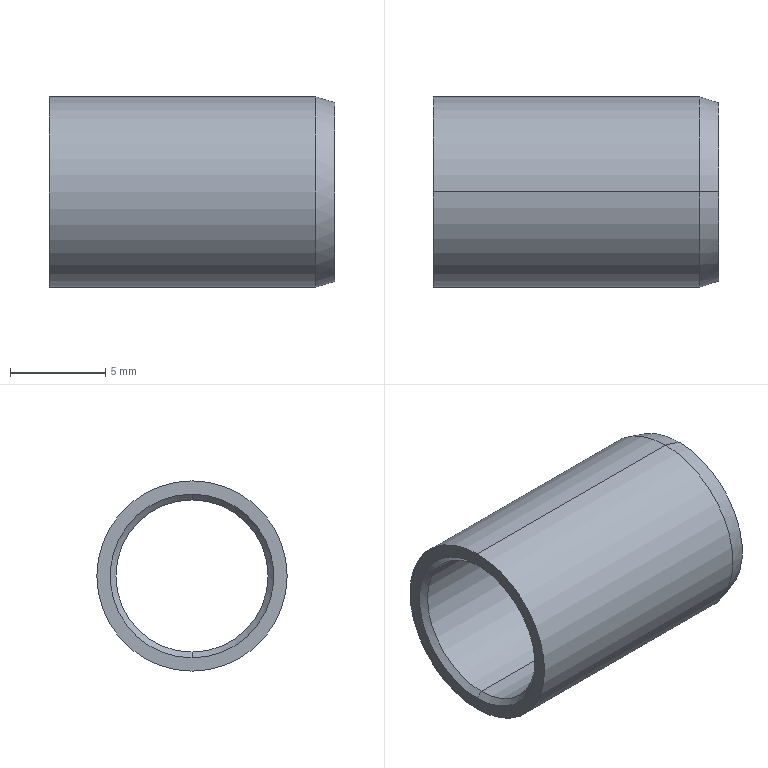Part | STEP file | 0246_001_JZB8-15 | 1 solid | 10 faces | box 15 x 10 x 10 mm | volume 418.338 mm3 | cylinder 4 | cone 4 | plane 2 | commonest cylinder face diameters 8 x2 10 x2
STEP:
#1=CARTESIAN_POINT('',(0.,0.,0.));
#2=DIRECTION('',(0.,0.,1.));
#3=DIRECTION('',(1.,0.,0.));
#4=AXIS2_PLACEMENT_3D('',#1,#2,#3);
#5=CARTESIAN_POINT('',(0.,0.,-5.));
#6=VERTEX_POINT('',#5);
#7=CARTESIAN_POINT('',(0.,0.,5.));
#8=VERTEX_POINT('',#7);
#9=CARTESIAN_POINT('',(0.,0.,0.));
#10=DIRECTION('',(1.,0.,0.));
#11=DIRECTION('',(0.,0.,-1.));
#12=AXIS2_PLACEMENT_3D('',#9,#10,#11);
#13=CIRCLE('',#12,5.);
#14=CARTESIAN_POINT('',(7.,0.,0.));
#15=DIRECTION('',(1.,0.,0.));
#16=DIRECTION('',(0.,0.,-1.));
#17=AXIS2_PLACEMENT_3D('',#14,#15,#16);
#18=CYLINDRICAL_SURFACE('',#17,5.);
#19=CARTESIAN_POINT('',(0.,-7.));
#20=DIRECTION('',(1.,0.));
#21=VECTOR('',#20,1.);
#22=LINE('',#19,#21);
#23=(GEOMETRIC_REPRESENTATION_CONTEXT(2)PARAMETRIC_REPRESENTATION_CONTEXT()REPRESENTATION_CONTEXT('',''));
#24=DEFINITIONAL_REPRESENTATION('',(#22),#23);
#25=PCURVE('',#18,#24);
#26=CARTESIAN_POINT('',(0.,4.65,0.));
#27=DIRECTION('',(-1.,0.,0.));
#28=DIRECTION('',(0.,0.,1.));
#29=AXIS2_PLACEMENT_3D('',#26,#27,#28);
#30=PLANE('',#29);
#31=CARTESIAN_POINT('',(-5.,-4.65));
#32=CARTESIAN_POINT('',(-5.,4.01));
#33=CARTESIAN_POINT('',(2.5,-0.3199));
#34=CARTESIAN_POINT('',(10.,-4.65));
#35=CARTESIAN_POINT('',(2.5,-8.98));
#36=CARTESIAN_POINT('',(-5.,-13.31));
#37=CARTESIAN_POINT('',(-5.,-4.65));
#38=(BOUNDED_CURVE()B_SPLINE_CURVE(2,(#31,#32,#33,#34,#35,#36,#37),.UNSPECIFIED.,.T.,.F.)B_SPLINE_CURVE_WITH_KNOTS((1,2,2,2,2,1),(-2.094,0.,2.094,4.189,6.283,8.378),.UNSPECIFIED.)CURVE()GEOMETRIC_REPRESENTATION_ITEM()RATIONAL_B_SPLINE_CURVE((1.,0.5,1.,0.5,1.,0.5,1.))REPRESENTATION_ITEM(''));
#39=(GEOMETRIC_REPRESENTATION_CONTEXT(2)PARAMETRIC_REPRESENTATION_CONTEXT()REPRESENTATION_CONTEXT('',''));
#40=DEFINITIONAL_REPRESENTATION('',(#38),#39);
#41=PCURVE('',#30,#40);
#42=SURFACE_CURVE('',#13,(#25,#41),.PCURVE_S1.);
#43=EDGE_CURVE('',#6,#8,#42,.T.);
#44=ORIENTED_EDGE('',*,*,#43,.T.);
#45=CARTESIAN_POINT('',(14.,0.,5.));
#46=VERTEX_POINT('',#45);
#47=CARTESIAN_POINT('',(7.,0.,5.));
#48=DIRECTION('',(1.,0.,0.));
#49=VECTOR('',#48,1.);
#50=LINE('',#47,#49);
#51=CARTESIAN_POINT('',(3.142,0.));
#52=DIRECTION('',(0.,1.));
#53=VECTOR('',#52,1.);
#54=LINE('',#51,#53);
#55=(GEOMETRIC_REPRESENTATION_CONTEXT(2)PARAMETRIC_REPRESENTATION_CONTEXT()REPRESENTATION_CONTEXT('',''));
#56=DEFINITIONAL_REPRESENTATION('',(#54),#55);
#57=PCURVE('',#18,#56);
#58=CARTESIAN_POINT('',(7.,0.,0.));
#59=DIRECTION('',(1.,0.,0.));
#60=DIRECTION('',(0.,0.,-1.));
#61=AXIS2_PLACEMENT_3D('',#58,#59,#60);
#62=CYLINDRICAL_SURFACE('',#61,5.);
#63=CARTESIAN_POINT('',(3.142,0.));
#64=DIRECTION('',(0.,1.));
#65=VECTOR('',#64,1.);
#66=LINE('',#63,#65);
#67=(GEOMETRIC_REPRESENTATION_CONTEXT(2)PARAMETRIC_REPRESENTATION_CONTEXT()REPRESENTATION_CONTEXT('',''));
#68=DEFINITIONAL_REPRESENTATION('',(#66),#67);
#69=PCURVE('',#62,#68);
#70=SURFACE_CURVE('',#50,(#57,#69),.PCURVE_S1.);
#71=EDGE_CURVE('',#8,#46,#70,.T.);
#72=ORIENTED_EDGE('',*,*,#71,.T.);
#73=CARTESIAN_POINT('',(14.,0.,-5.));
#74=VERTEX_POINT('',#73);
#75=CARTESIAN_POINT('',(14.,0.,0.));
#76=DIRECTION('',(-1.,0.,0.));
#77=DIRECTION('',(0.,0.,-1.));
#78=AXIS2_PLACEMENT_3D('',#75,#76,#77);
#79=CIRCLE('',#78,5.);
#80=CARTESIAN_POINT('',(6.283,7.));
#81=DIRECTION('',(-1.,0.));
#82=VECTOR('',#81,1.);
#83=LINE('',#80,#82);
#84=(GEOMETRIC_REPRESENTATION_CONTEXT(2)PARAMETRIC_REPRESENTATION_CONTEXT()REPRESENTATION_CONTEXT('',''));
#85=DEFINITIONAL_REPRESENTATION('',(#83),#84);
#86=PCURVE('',#18,#85);
#87=CARTESIAN_POINT('',(14.,0.,0.));
#88=DIRECTION('',(-1.,0.,0.));
#89=DIRECTION('',(0.,0.,1.));
#90=AXIS2_PLACEMENT_3D('',#87,#88,#89);
#91=CONICAL_SURFACE('',#90,5.,0.2915);
#92=CARTESIAN_POINT('',(-3.142,0.));
#93=DIRECTION('',(1.,0.));
#94=VECTOR('',#93,1.);
#95=LINE('',#92,#94);
#96=(GEOMETRIC_REPRESENTATION_CONTEXT(2)PARAMETRIC_REPRESENTATION_CONTEXT()REPRESENTATION_CONTEXT('',''));
#97=DEFINITIONAL_REPRESENTATION('',(#95),#96);
#98=PCURVE('',#91,#97);
#99=SURFACE_CURVE('',#79,(#86,#98),.PCURVE_S1.);
#100=EDGE_CURVE('',#46,#74,#99,.T.);
#101=ORIENTED_EDGE('',*,*,#100,.T.);
#102=CARTESIAN_POINT('',(7.,0.,-5.));
#103=DIRECTION('',(1.,0.,0.));
#104=VECTOR('',#103,1.);
#105=LINE('',#102,#104);
#106=CARTESIAN_POINT('',(0.,0.));
#107=DIRECTION('',(0.,1.));
#108=VECTOR('',#107,1.);
#109=LINE('',#106,#108);
#110=(GEOMETRIC_REPRESENTATION_CONTEXT(2)PARAMETRIC_REPRESENTATION_CONTEXT()REPRESENTATION_CONTEXT('',''));
#111=DEFINITIONAL_REPRESENTATION('',(#109),#110);
#112=PCURVE('',#18,#111);
#113=CARTESIAN_POINT('',(6.283,0.));
#114=DIRECTION('',(0.,1.));
#115=VECTOR('',#114,1.);
#116=LINE('',#113,#115);
#117=(GEOMETRIC_REPRESENTATION_CONTEXT(2)PARAMETRIC_REPRESENTATION_CONTEXT()REPRESENTATION_CONTEXT('',''));
#118=DEFINITIONAL_REPRESENTATION('',(#116),#117);
#119=PCURVE('',#62,#118);
#120=SURFACE_CURVE('',#105,(#112,#119),.PCURVE_S1.);
#121=EDGE_CURVE('',#6,#74,#120,.T.);
#122=ORIENTED_EDGE('',*,*,#121,.F.);
#123=EDGE_LOOP('',(#44,#72,#101,#122));
#124=FACE_BOUND('',#123,.T.);
#125=ADVANCED_FACE('',(#124),#18,.T.);
#126=CARTESIAN_POINT('',(15.,0.,4.7));
#127=VERTEX_POINT('',#126);
#128=CARTESIAN_POINT('',(15.,0.,-4.7));
#129=VERTEX_POINT('',#128);
#130=CARTESIAN_POINT('',(15.,0.,0.));
#131=DIRECTION('',(-1.,0.,0.));
#132=DIRECTION('',(0.,0.,1.));
#133=AXIS2_PLACEMENT_3D('',#130,#131,#132);
#134=CIRCLE('',#133,4.7);
#135=CARTESIAN_POINT('',(0.,-1.));
#136=DIRECTION('',(1.,0.));
#137=VECTOR('',#136,1.);
#138=LINE('',#135,#137);
#139=(GEOMETRIC_REPRESENTATION_CONTEXT(2)PARAMETRIC_REPRESENTATION_CONTEXT()REPRESENTATION_CONTEXT('',''));
#140=DEFINITIONAL_REPRESENTATION('',(#138),#139);
#141=PCURVE('',#91,#140);
#142=CARTESIAN_POINT('',(15.,4.35,0.));
#143=DIRECTION('',(1.,0.,0.));
#144=DIRECTION('',(0.,0.,-1.));
#145=AXIS2_PLACEMENT_3D('',#142,#143,#144);
#146=PLANE('',#145);
#147=CARTESIAN_POINT('',(-4.7,-4.35));
#148=CARTESIAN_POINT('',(-4.7,3.791));
#149=CARTESIAN_POINT('',(2.35,-0.2797));
#150=CARTESIAN_POINT('',(9.4,-4.35));
#151=CARTESIAN_POINT('',(2.35,-8.42));
#152=CARTESIAN_POINT('',(-4.7,-12.491));
#153=CARTESIAN_POINT('',(-4.7,-4.35));
#154=(BOUNDED_CURVE()B_SPLINE_CURVE(2,(#147,#148,#149,#150,#151,#152,#153),.UNSPECIFIED.,.T.,.F.)B_SPLINE_CURVE_WITH_KNOTS((1,2,2,2,2,1),(-2.094,0.,2.094,4.189,6.283,8.378),.UNSPECIFIED.)CURVE()GEOMETRIC_REPRESENTATION_ITEM()RATIONAL_B_SPLINE_CURVE((1.,0.5,1.,0.5,1.,0.5,1.))REPRESENTATION_ITEM(''));
#155=(GEOMETRIC_REPRESENTATION_CONTEXT(2)PARAMETRIC_REPRESENTATION_CONTEXT()REPRESENTATION_CONTEXT('',''));
#156=DEFINITIONAL_REPRESENTATION('',(#154),#155);
#157=PCURVE('',#146,#156);
#158=SURFACE_CURVE('',#134,(#141,#157),.PCURVE_S1.);
#159=EDGE_CURVE('',#127,#129,#158,.T.);
#160=ORIENTED_EDGE('',*,*,#159,.T.);
#161=CARTESIAN_POINT('',(14.,0.,-5.));
#162=DIRECTION('',(-0.9578,0.,-0.2873));
#163=VECTOR('',#162,1.);
#164=LINE('',#161,#163);
#165=CARTESIAN_POINT('',(3.142,0.));
#166=DIRECTION('',(0.,1.));
#167=VECTOR('',#166,1.);
#168=LINE('',#165,#167);
#169=(GEOMETRIC_REPRESENTATION_CONTEXT(2)PARAMETRIC_REPRESENTATION_CONTEXT()REPRESENTATION_CONTEXT('',''));
#170=DEFINITIONAL_REPRESENTATION('',(#168),#169);
#171=PCURVE('',#91,#170);
#172=CARTESIAN_POINT('',(14.,0.,0.));
#173=DIRECTION('',(-1.,0.,0.));
#174=DIRECTION('',(0.,0.,1.));
#175=AXIS2_PLACEMENT_3D('',#172,#173,#174);
#176=CONICAL_SURFACE('',#175,5.,0.2915);
#177=CARTESIAN_POINT('',(3.142,0.));
#178=DIRECTION('',(0.,1.));
#179=VECTOR('',#178,1.);
#180=LINE('',#177,#179);
#181=(GEOMETRIC_REPRESENTATION_CONTEXT(2)PARAMETRIC_REPRESENTATION_CONTEXT()REPRESENTATION_CONTEXT('',''));
#182=DEFINITIONAL_REPRESENTATION('',(#180),#181);
#183=PCURVE('',#176,#182);
#184=SURFACE_CURVE('',#164,(#171,#183),.PCURVE_S1.);
#185=EDGE_CURVE('',#129,#74,#184,.T.);
#186=ORIENTED_EDGE('',*,*,#185,.T.);
#187=ORIENTED_EDGE('',*,*,#100,.F.);
#188=CARTESIAN_POINT('',(14.,0.,5.));
#189=DIRECTION('',(-0.9578,0.,0.2873));
#190=VECTOR('',#189,1.);
#191=LINE('',#188,#190);
#192=CARTESIAN_POINT('',(0.,0.));
#193=DIRECTION('',(0.,1.));
#194=VECTOR('',#193,1.);
#195=LINE('',#192,#194);
#196=(GEOMETRIC_REPRESENTATION_CONTEXT(2)PARAMETRIC_REPRESENTATION_CONTEXT()REPRESENTATION_CONTEXT('',''));
#197=DEFINITIONAL_REPRESENTATION('',(#195),#196);
#198=PCURVE('',#91,#197);
#199=CARTESIAN_POINT('',(6.283,0.));
#200=DIRECTION('',(0.,1.));
#201=VECTOR('',#200,1.);
#202=LINE('',#199,#201);
#203=(GEOMETRIC_REPRESENTATION_CONTEXT(2)PARAMETRIC_REPRESENTATION_CONTEXT()REPRESENTATION_CONTEXT('',''));
#204=DEFINITIONAL_REPRESENTATION('',(#202),#203);
#205=PCURVE('',#176,#204);
#206=SURFACE_CURVE('',#191,(#198,#205),.PCURVE_S1.);
#207=EDGE_CURVE('',#127,#46,#206,.T.);
#208=ORIENTED_EDGE('',*,*,#207,.F.);
#209=EDGE_LOOP('',(#160,#186,#187,#208));
#210=FACE_BOUND('',#209,.T.);
#211=ADVANCED_FACE('',(#210),#91,.T.);
#212=CARTESIAN_POINT('',(0.3,0.,4.));
#213=VERTEX_POINT('',#212);
#214=CARTESIAN_POINT('',(0.,0.,4.3));
#215=VERTEX_POINT('',#214);
#216=CARTESIAN_POINT('',(0.,0.,4.3));
#217=DIRECTION('',(-0.7071,0.,0.7071));
#218=VECTOR('',#217,1.);
#219=LINE('',#216,#218);
#220=CARTESIAN_POINT('',(0.,0.,0.));
#221=DIRECTION('',(-1.,0.,0.));
#222=DIRECTION('',(0.,0.,1.));
#223=AXIS2_PLACEMENT_3D('',#220,#221,#222);
#224=CONICAL_SURFACE('',#223,4.3,0.7854);
#225=CARTESIAN_POINT('',(6.283,0.));
#226=DIRECTION('',(0.,1.));
#227=VECTOR('',#226,1.);
#228=LINE('',#225,#227);
#229=(GEOMETRIC_REPRESENTATION_CONTEXT(2)PARAMETRIC_REPRESENTATION_CONTEXT()REPRESENTATION_CONTEXT('',''));
#230=DEFINITIONAL_REPRESENTATION('',(#228),#229);
#231=PCURVE('',#224,#230);
#232=CARTESIAN_POINT('',(0.,0.,0.));
#233=DIRECTION('',(-1.,0.,0.));
#234=DIRECTION('',(0.,0.,1.));
#235=AXIS2_PLACEMENT_3D('',#232,#233,#234);
#236=CONICAL_SURFACE('',#235,4.3,0.7854);
#237=CARTESIAN_POINT('',(0.,0.));
#238=DIRECTION('',(0.,1.));
#239=VECTOR('',#238,1.);
#240=LINE('',#237,#239);
#241=(GEOMETRIC_REPRESENTATION_CONTEXT(2)PARAMETRIC_REPRESENTATION_CONTEXT()REPRESENTATION_CONTEXT('',''));
#242=DEFINITIONAL_REPRESENTATION('',(#240),#241);
#243=PCURVE('',#236,#242);
#244=SURFACE_CURVE('',#219,(#231,#243),.PCURVE_S1.);
#245=EDGE_CURVE('',#213,#215,#244,.T.);
#246=ORIENTED_EDGE('',*,*,#245,.T.);
#247=CARTESIAN_POINT('',(0.,0.,-4.3));
#248=VERTEX_POINT('',#247);
#249=CARTESIAN_POINT('',(0.,0.,0.));
#250=DIRECTION('',(1.,0.,0.));
#251=DIRECTION('',(0.,0.,1.));
#252=AXIS2_PLACEMENT_3D('',#249,#250,#251);
#253=CIRCLE('',#252,4.3);
#254=CARTESIAN_POINT('',(6.283,0.));
#255=DIRECTION('',(-1.,0.));
#256=VECTOR('',#255,1.);
#257=LINE('',#254,#256);
#258=(GEOMETRIC_REPRESENTATION_CONTEXT(2)PARAMETRIC_REPRESENTATION_CONTEXT()REPRESENTATION_CONTEXT('',''));
#259=DEFINITIONAL_REPRESENTATION('',(#257),#258);
#260=PCURVE('',#224,#259);
#261=CARTESIAN_POINT('',(4.3,-4.65));
#262=CARTESIAN_POINT('',(4.3,-12.098));
#263=CARTESIAN_POINT('',(-2.15,-8.374));
#264=CARTESIAN_POINT('',(-8.6,-4.65));
#265=CARTESIAN_POINT('',(-2.15,-0.9261));
#266=CARTESIAN_POINT('',(4.3,2.798));
#267=CARTESIAN_POINT('',(4.3,-4.65));
#268=(BOUNDED_CURVE()B_SPLINE_CURVE(2,(#261,#262,#263,#264,#265,#266,#267),.UNSPECIFIED.,.T.,.F.)B_SPLINE_CURVE_WITH_KNOTS((1,2,2,2,2,1),(-2.094,0.,2.094,4.189,6.283,8.378),.UNSPECIFIED.)CURVE()GEOMETRIC_REPRESENTATION_ITEM()RATIONAL_B_SPLINE_CURVE((1.,0.5,1.,0.5,1.,0.5,1.))REPRESENTATION_ITEM(''));
#269=(GEOMETRIC_REPRESENTATION_CONTEXT(2)PARAMETRIC_REPRESENTATION_CONTEXT()REPRESENTATION_CONTEXT('',''));
#270=DEFINITIONAL_REPRESENTATION('',(#268),#269);
#271=PCURVE('',#30,#270);
#272=SURFACE_CURVE('',#253,(#260,#271),.PCURVE_S1.);
#273=EDGE_CURVE('',#215,#248,#272,.T.);
#274=ORIENTED_EDGE('',*,*,#273,.T.);
#275=CARTESIAN_POINT('',(0.3,0.,-4.));
#276=VERTEX_POINT('',#275);
#277=CARTESIAN_POINT('',(0.,0.,-4.3));
#278=DIRECTION('',(-0.7071,0.,-0.7071));
#279=VECTOR('',#278,1.);
#280=LINE('',#277,#279);
#281=CARTESIAN_POINT('',(3.142,0.));
#282=DIRECTION('',(0.,1.));
#283=VECTOR('',#282,1.);
#284=LINE('',#281,#283);
#285=(GEOMETRIC_REPRESENTATION_CONTEXT(2)PARAMETRIC_REPRESENTATION_CONTEXT()REPRESENTATION_CONTEXT('',''));
#286=DEFINITIONAL_REPRESENTATION('',(#284),#285);
#287=PCURVE('',#224,#286);
#288=CARTESIAN_POINT('',(3.142,0.));
#289=DIRECTION('',(0.,1.));
#290=VECTOR('',#289,1.);
#291=LINE('',#288,#290);
#292=(GEOMETRIC_REPRESENTATION_CONTEXT(2)PARAMETRIC_REPRESENTATION_CONTEXT()REPRESENTATION_CONTEXT('',''));
#293=DEFINITIONAL_REPRESENTATION('',(#291),#292);
#294=PCURVE('',#236,#293);
#295=SURFACE_CURVE('',#280,(#287,#294),.PCURVE_S1.);
#296=EDGE_CURVE('',#276,#248,#295,.T.);
#297=ORIENTED_EDGE('',*,*,#296,.F.);
#298=CARTESIAN_POINT('',(0.3,0.,0.));
#299=DIRECTION('',(-1.,0.,0.));
#300=DIRECTION('',(0.,1.,0.));
#301=AXIS2_PLACEMENT_3D('',#298,#299,#300);
#302=CIRCLE('',#301,4.);
#303=CARTESIAN_POINT('',(1.571,-0.3));
#304=DIRECTION('',(1.,0.));
#305=VECTOR('',#304,1.);
#306=LINE('',#303,#305);
#307=(GEOMETRIC_REPRESENTATION_CONTEXT(2)PARAMETRIC_REPRESENTATION_CONTEXT()REPRESENTATION_CONTEXT('',''));
#308=DEFINITIONAL_REPRESENTATION('',(#306),#307);
#309=PCURVE('',#224,#308);
#310=CARTESIAN_POINT('',(7.65,0.,0.));
#311=DIRECTION('',(1.,0.,0.));
#312=DIRECTION('',(0.,0.,-1.));
#313=AXIS2_PLACEMENT_3D('',#310,#311,#312);
#314=CYLINDRICAL_SURFACE('',#313,4.);
#315=CARTESIAN_POINT('',(7.854,-7.35));
#316=DIRECTION('',(-1.,0.));
#317=VECTOR('',#316,1.);
#318=LINE('',#315,#317);
#319=(GEOMETRIC_REPRESENTATION_CONTEXT(2)PARAMETRIC_REPRESENTATION_CONTEXT()REPRESENTATION_CONTEXT('',''));
#320=DEFINITIONAL_REPRESENTATION('',(#318),#319);
#321=PCURVE('',#314,#320);
#322=SURFACE_CURVE('',#302,(#309,#321),.PCURVE_S1.);
#323=EDGE_CURVE('',#276,#213,#322,.T.);
#324=ORIENTED_EDGE('',*,*,#323,.T.);
#325=EDGE_LOOP('',(#246,#274,#297,#324));
#326=FACE_BOUND('',#325,.F.);
#327=ADVANCED_FACE('',(#326),#224,.F.);
#328=CARTESIAN_POINT('',(15.,0.,-4.));
#329=VERTEX_POINT('',#328);
#330=CARTESIAN_POINT('',(7.65,0.,-4.));
#331=DIRECTION('',(1.,0.,0.));
#332=VECTOR('',#331,1.);
#333=LINE('',#330,#332);
#334=CARTESIAN_POINT('',(6.283,0.));
#335=DIRECTION('',(0.,1.));
#336=VECTOR('',#335,1.);
#337=LINE('',#334,#336);
#338=(GEOMETRIC_REPRESENTATION_CONTEXT(2)PARAMETRIC_REPRESENTATION_CONTEXT()REPRESENTATION_CONTEXT('',''));
#339=DEFINITIONAL_REPRESENTATION('',(#337),#338);
#340=PCURVE('',#314,#339);
#341=CARTESIAN_POINT('',(7.65,0.,0.));
#342=DIRECTION('',(1.,0.,0.));
#343=DIRECTION('',(0.,0.,-1.));
#344=AXIS2_PLACEMENT_3D('',#341,#342,#343);
#345=CYLINDRICAL_SURFACE('',#344,4.);
#346=CARTESIAN_POINT('',(0.,0.));
#347=DIRECTION('',(0.,1.));
#348=VECTOR('',#347,1.);
#349=LINE('',#346,#348);
#350=(GEOMETRIC_REPRESENTATION_CONTEXT(2)PARAMETRIC_REPRESENTATION_CONTEXT()REPRESENTATION_CONTEXT('',''));
#351=DEFINITIONAL_REPRESENTATION('',(#349),#350);
#352=PCURVE('',#345,#351);
#353=SURFACE_CURVE('',#333,(#340,#352),.PCURVE_S1.);
#354=EDGE_CURVE('',#276,#329,#353,.T.);
#355=ORIENTED_EDGE('',*,*,#354,.T.);
#356=CARTESIAN_POINT('',(15.,0.,4.));
#357=VERTEX_POINT('',#356);
#358=CARTESIAN_POINT('',(15.,0.,0.));
#359=DIRECTION('',(-1.,0.,0.));
#360=DIRECTION('',(0.,0.,-1.));
#361=AXIS2_PLACEMENT_3D('',#358,#359,#360);
#362=CIRCLE('',#361,4.);
#363=CARTESIAN_POINT('',(6.283,7.35));
#364=DIRECTION('',(-1.,0.));
#365=VECTOR('',#364,1.);
#366=LINE('',#363,#365);
#367=(GEOMETRIC_REPRESENTATION_CONTEXT(2)PARAMETRIC_REPRESENTATION_CONTEXT()REPRESENTATION_CONTEXT('',''));
#368=DEFINITIONAL_REPRESENTATION('',(#366),#367);
#369=PCURVE('',#314,#368);
#370=CARTESIAN_POINT('',(4.,-4.35));
#371=CARTESIAN_POINT('',(4.,-11.278));
#372=CARTESIAN_POINT('',(-2.,-7.814));
#373=CARTESIAN_POINT('',(-8.,-4.35));
#374=CARTESIAN_POINT('',(-2.,-0.8859));
#375=CARTESIAN_POINT('',(4.,2.578));
#376=CARTESIAN_POINT('',(4.,-4.35));
#377=(BOUNDED_CURVE()B_SPLINE_CURVE(2,(#370,#371,#372,#373,#374,#375,#376),.UNSPECIFIED.,.T.,.F.)B_SPLINE_CURVE_WITH_KNOTS((1,2,2,2,2,1),(-2.094,0.,2.094,4.189,6.283,8.378),.UNSPECIFIED.)CURVE()GEOMETRIC_REPRESENTATION_ITEM()RATIONAL_B_SPLINE_CURVE((1.,0.5,1.,0.5,1.,0.5,1.))REPRESENTATION_ITEM(''));
#378=(GEOMETRIC_REPRESENTATION_CONTEXT(2)PARAMETRIC_REPRESENTATION_CONTEXT()REPRESENTATION_CONTEXT('',''));
#379=DEFINITIONAL_REPRESENTATION('',(#377),#378);
#380=PCURVE('',#146,#379);
#381=SURFACE_CURVE('',#362,(#369,#380),.PCURVE_S1.);
#382=EDGE_CURVE('',#329,#357,#381,.T.);
#383=ORIENTED_EDGE('',*,*,#382,.T.);
#384=CARTESIAN_POINT('',(7.65,0.,4.));
#385=DIRECTION('',(1.,0.,0.));
#386=VECTOR('',#385,1.);
#387=LINE('',#384,#386);
#388=CARTESIAN_POINT('',(3.142,0.));
#389=DIRECTION('',(0.,1.));
#390=VECTOR('',#389,1.);
#391=LINE('',#388,#390);
#392=(GEOMETRIC_REPRESENTATION_CONTEXT(2)PARAMETRIC_REPRESENTATION_CONTEXT()REPRESENTATION_CONTEXT('',''));
#393=DEFINITIONAL_REPRESENTATION('',(#391),#392);
#394=PCURVE('',#314,#393);
#395=CARTESIAN_POINT('',(3.142,0.));
#396=DIRECTION('',(0.,1.));
#397=VECTOR('',#396,1.);
#398=LINE('',#395,#397);
#399=(GEOMETRIC_REPRESENTATION_CONTEXT(2)PARAMETRIC_REPRESENTATION_CONTEXT()REPRESENTATION_CONTEXT('',''));
#400=DEFINITIONAL_REPRESENTATION('',(#398),#399);
#401=PCURVE('',#345,#400);
#402=SURFACE_CURVE('',#387,(#394,#401),.PCURVE_S1.);
#403=EDGE_CURVE('',#213,#357,#402,.T.);
#404=ORIENTED_EDGE('',*,*,#403,.F.);
#405=ORIENTED_EDGE('',*,*,#323,.F.);
#406=EDGE_LOOP('',(#355,#383,#404,#405));
#407=FACE_BOUND('',#406,.F.);
#408=ADVANCED_FACE('',(#407),#314,.F.);
#409=ORIENTED_EDGE('',*,*,#71,.F.);
#410=CARTESIAN_POINT('',(0.,0.,0.));
#411=DIRECTION('',(1.,0.,0.));
#412=DIRECTION('',(0.,0.,-1.));
#413=AXIS2_PLACEMENT_3D('',#410,#411,#412);
#414=CIRCLE('',#413,5.);
#415=CARTESIAN_POINT('',(0.,-7.));
#416=DIRECTION('',(1.,0.));
#417=VECTOR('',#416,1.);
#418=LINE('',#415,#417);
#419=(GEOMETRIC_REPRESENTATION_CONTEXT(2)PARAMETRIC_REPRESENTATION_CONTEXT()REPRESENTATION_CONTEXT('',''));
#420=DEFINITIONAL_REPRESENTATION('',(#418),#419);
#421=PCURVE('',#62,#420);
#422=CARTESIAN_POINT('',(-5.,-4.65));
#423=CARTESIAN_POINT('',(-5.,4.01));
#424=CARTESIAN_POINT('',(2.5,-0.3199));
#425=CARTESIAN_POINT('',(10.,-4.65));
#426=CARTESIAN_POINT('',(2.5,-8.98));
#427=CARTESIAN_POINT('',(-5.,-13.31));
#428=CARTESIAN_POINT('',(-5.,-4.65));
#429=(BOUNDED_CURVE()B_SPLINE_CURVE(2,(#422,#423,#424,#425,#426,#427,#428),.UNSPECIFIED.,.T.,.F.)B_SPLINE_CURVE_WITH_KNOTS((1,2,2,2,2,1),(-2.094,0.,2.094,4.189,6.283,8.378),.UNSPECIFIED.)CURVE()GEOMETRIC_REPRESENTATION_ITEM()RATIONAL_B_SPLINE_CURVE((1.,0.5,1.,0.5,1.,0.5,1.))REPRESENTATION_ITEM(''));
#430=(GEOMETRIC_REPRESENTATION_CONTEXT(2)PARAMETRIC_REPRESENTATION_CONTEXT()REPRESENTATION_CONTEXT('',''));
#431=DEFINITIONAL_REPRESENTATION('',(#429),#430);
#432=PCURVE('',#30,#431);
#433=SURFACE_CURVE('',#414,(#421,#432),.PCURVE_S1.);
#434=EDGE_CURVE('',#8,#6,#433,.T.);
#435=ORIENTED_EDGE('',*,*,#434,.T.);
#436=ORIENTED_EDGE('',*,*,#121,.T.);
#437=CARTESIAN_POINT('',(14.,0.,0.));
#438=DIRECTION('',(-1.,0.,0.));
#439=DIRECTION('',(0.,0.,-1.));
#440=AXIS2_PLACEMENT_3D('',#437,#438,#439);
#441=CIRCLE('',#440,5.);
#442=CARTESIAN_POINT('',(6.283,7.));
#443=DIRECTION('',(-1.,0.));
#444=VECTOR('',#443,1.);
#445=LINE('',#442,#444);
#446=(GEOMETRIC_REPRESENTATION_CONTEXT(2)PARAMETRIC_REPRESENTATION_CONTEXT()REPRESENTATION_CONTEXT('',''));
#447=DEFINITIONAL_REPRESENTATION('',(#445),#446);
#448=PCURVE('',#62,#447);
#449=CARTESIAN_POINT('',(3.142,0.));
#450=DIRECTION('',(1.,0.));
#451=VECTOR('',#450,1.);
#452=LINE('',#449,#451);
#453=(GEOMETRIC_REPRESENTATION_CONTEXT(2)PARAMETRIC_REPRESENTATION_CONTEXT()REPRESENTATION_CONTEXT('',''));
#454=DEFINITIONAL_REPRESENTATION('',(#452),#453);
#455=PCURVE('',#176,#454);
#456=SURFACE_CURVE('',#441,(#448,#455),.PCURVE_S1.);
#457=EDGE_CURVE('',#74,#46,#456,.T.);
#458=ORIENTED_EDGE('',*,*,#457,.T.);
#459=EDGE_LOOP('',(#409,#435,#436,#458));
#460=FACE_BOUND('',#459,.T.);
#461=ADVANCED_FACE('',(#460),#62,.T.);
#462=ORIENTED_EDGE('',*,*,#43,.F.);
#463=ORIENTED_EDGE('',*,*,#434,.F.);
#464=EDGE_LOOP('',(#462,#463));
#465=FACE_BOUND('',#464,.T.);
#466=ORIENTED_EDGE('',*,*,#273,.T.);
#467=CARTESIAN_POINT('',(0.,0.,0.));
#468=DIRECTION('',(1.,0.,0.));
#469=DIRECTION('',(0.,0.,1.));
#470=AXIS2_PLACEMENT_3D('',#467,#468,#469);
#471=CIRCLE('',#470,4.3);
#472=CARTESIAN_POINT('',(4.3,-4.65));
#473=CARTESIAN_POINT('',(4.3,-12.098));
#474=CARTESIAN_POINT('',(-2.15,-8.374));
#475=CARTESIAN_POINT('',(-8.6,-4.65));
#476=CARTESIAN_POINT('',(-2.15,-0.9261));
#477=CARTESIAN_POINT('',(4.3,2.798));
#478=CARTESIAN_POINT('',(4.3,-4.65));
#479=(BOUNDED_CURVE()B_SPLINE_CURVE(2,(#472,#473,#474,#475,#476,#477,#478),.UNSPECIFIED.,.T.,.F.)B_SPLINE_CURVE_WITH_KNOTS((1,2,2,2,2,1),(-2.094,0.,2.094,4.189,6.283,8.378),.UNSPECIFIED.)CURVE()GEOMETRIC_REPRESENTATION_ITEM()RATIONAL_B_SPLINE_CURVE((1.,0.5,1.,0.5,1.,0.5,1.))REPRESENTATION_ITEM(''));
#480=(GEOMETRIC_REPRESENTATION_CONTEXT(2)PARAMETRIC_REPRESENTATION_CONTEXT()REPRESENTATION_CONTEXT('',''));
#481=DEFINITIONAL_REPRESENTATION('',(#479),#480);
#482=PCURVE('',#30,#481);
#483=CARTESIAN_POINT('',(6.283,0.));
#484=DIRECTION('',(-1.,0.));
#485=VECTOR('',#484,1.);
#486=LINE('',#483,#485);
#487=(GEOMETRIC_REPRESENTATION_CONTEXT(2)PARAMETRIC_REPRESENTATION_CONTEXT()REPRESENTATION_CONTEXT('',''));
#488=DEFINITIONAL_REPRESENTATION('',(#486),#487);
#489=PCURVE('',#236,#488);
#490=SURFACE_CURVE('',#471,(#482,#489),.PCURVE_S1.);
#491=EDGE_CURVE('',#248,#215,#490,.T.);
#492=ORIENTED_EDGE('',*,*,#491,.T.);
#493=EDGE_LOOP('',(#466,#492));
#494=FACE_BOUND('',#493,.T.);
#495=ADVANCED_FACE('',(#465,#494),#30,.T.);
#496=ORIENTED_EDGE('',*,*,#185,.F.);
#497=CARTESIAN_POINT('',(15.,0.,0.));
#498=DIRECTION('',(-1.,0.,0.));
#499=DIRECTION('',(0.,0.,1.));
#500=AXIS2_PLACEMENT_3D('',#497,#498,#499);
#501=CIRCLE('',#500,4.7);
#502=CARTESIAN_POINT('',(0.,-1.));
#503=DIRECTION('',(1.,0.));
#504=VECTOR('',#503,1.);
#505=LINE('',#502,#504);
#506=(GEOMETRIC_REPRESENTATION_CONTEXT(2)PARAMETRIC_REPRESENTATION_CONTEXT()REPRESENTATION_CONTEXT('',''));
#507=DEFINITIONAL_REPRESENTATION('',(#505),#506);
#508=PCURVE('',#176,#507);
#509=CARTESIAN_POINT('',(-4.7,-4.35));
#510=CARTESIAN_POINT('',(-4.7,3.791));
#511=CARTESIAN_POINT('',(2.35,-0.2797));
#512=CARTESIAN_POINT('',(9.4,-4.35));
#513=CARTESIAN_POINT('',(2.35,-8.42));
#514=CARTESIAN_POINT('',(-4.7,-12.491));
#515=CARTESIAN_POINT('',(-4.7,-4.35));
#516=(BOUNDED_CURVE()B_SPLINE_CURVE(2,(#509,#510,#511,#512,#513,#514,#515),.UNSPECIFIED.,.T.,.F.)B_SPLINE_CURVE_WITH_KNOTS((1,2,2,2,2,1),(-2.094,0.,2.094,4.189,6.283,8.378),.UNSPECIFIED.)CURVE()GEOMETRIC_REPRESENTATION_ITEM()RATIONAL_B_SPLINE_CURVE((1.,0.5,1.,0.5,1.,0.5,1.))REPRESENTATION_ITEM(''));
#517=(GEOMETRIC_REPRESENTATION_CONTEXT(2)PARAMETRIC_REPRESENTATION_CONTEXT()REPRESENTATION_CONTEXT('',''));
#518=DEFINITIONAL_REPRESENTATION('',(#516),#517);
#519=PCURVE('',#146,#518);
#520=SURFACE_CURVE('',#501,(#508,#519),.PCURVE_S1.);
#521=EDGE_CURVE('',#129,#127,#520,.T.);
#522=ORIENTED_EDGE('',*,*,#521,.T.);
#523=ORIENTED_EDGE('',*,*,#207,.T.);
#524=ORIENTED_EDGE('',*,*,#457,.F.);
#525=EDGE_LOOP('',(#496,#522,#523,#524));
#526=FACE_BOUND('',#525,.T.);
#527=ADVANCED_FACE('',(#526),#176,.T.);
#528=ORIENTED_EDGE('',*,*,#491,.T.);
#529=ORIENTED_EDGE('',*,*,#245,.F.);
#530=CARTESIAN_POINT('',(0.3,0.,0.));
#531=DIRECTION('',(-1.,0.,0.));
#532=DIRECTION('',(0.,1.,0.));
#533=AXIS2_PLACEMENT_3D('',#530,#531,#532);
#534=CIRCLE('',#533,4.);
#535=CARTESIAN_POINT('',(-4.712,-0.3));
#536=DIRECTION('',(1.,0.));
#537=VECTOR('',#536,1.);
#538=LINE('',#535,#537);
#539=(GEOMETRIC_REPRESENTATION_CONTEXT(2)PARAMETRIC_REPRESENTATION_CONTEXT()REPRESENTATION_CONTEXT('',''));
#540=DEFINITIONAL_REPRESENTATION('',(#538),#539);
#541=PCURVE('',#236,#540);
#542=CARTESIAN_POINT('',(7.854,-7.35));
#543=DIRECTION('',(-1.,0.));
#544=VECTOR('',#543,1.);
#545=LINE('',#542,#544);
#546=(GEOMETRIC_REPRESENTATION_CONTEXT(2)PARAMETRIC_REPRESENTATION_CONTEXT()REPRESENTATION_CONTEXT('',''));
#547=DEFINITIONAL_REPRESENTATION('',(#545),#546);
#548=PCURVE('',#345,#547);
#549=SURFACE_CURVE('',#534,(#541,#548),.PCURVE_S1.);
#550=EDGE_CURVE('',#213,#276,#549,.T.);
#551=ORIENTED_EDGE('',*,*,#550,.T.);
#552=ORIENTED_EDGE('',*,*,#296,.T.);
#553=EDGE_LOOP('',(#528,#529,#551,#552));
#554=FACE_BOUND('',#553,.F.);
#555=ADVANCED_FACE('',(#554),#236,.F.);
#556=ORIENTED_EDGE('',*,*,#382,.T.);
#557=CARTESIAN_POINT('',(15.,0.,0.));
#558=DIRECTION('',(-1.,0.,0.));
#559=DIRECTION('',(0.,0.,-1.));
#560=AXIS2_PLACEMENT_3D('',#557,#558,#559);
#561=CIRCLE('',#560,4.);
#562=CARTESIAN_POINT('',(4.,-4.35));
#563=CARTESIAN_POINT('',(4.,-11.278));
#564=CARTESIAN_POINT('',(-2.,-7.814));
#565=CARTESIAN_POINT('',(-8.,-4.35));
#566=CARTESIAN_POINT('',(-2.,-0.8859));
#567=CARTESIAN_POINT('',(4.,2.578));
#568=CARTESIAN_POINT('',(4.,-4.35));
#569=(BOUNDED_CURVE()B_SPLINE_CURVE(2,(#562,#563,#564,#565,#566,#567,#568),.UNSPECIFIED.,.T.,.F.)B_SPLINE_CURVE_WITH_KNOTS((1,2,2,2,2,1),(-2.094,0.,2.094,4.189,6.283,8.378),.UNSPECIFIED.)CURVE()GEOMETRIC_REPRESENTATION_ITEM()RATIONAL_B_SPLINE_CURVE((1.,0.5,1.,0.5,1.,0.5,1.))REPRESENTATION_ITEM(''));
#570=(GEOMETRIC_REPRESENTATION_CONTEXT(2)PARAMETRIC_REPRESENTATION_CONTEXT()REPRESENTATION_CONTEXT('',''));
#571=DEFINITIONAL_REPRESENTATION('',(#569),#570);
#572=PCURVE('',#146,#571);
#573=CARTESIAN_POINT('',(6.283,7.35));
#574=DIRECTION('',(-1.,0.));
#575=VECTOR('',#574,1.);
#576=LINE('',#573,#575);
#577=(GEOMETRIC_REPRESENTATION_CONTEXT(2)PARAMETRIC_REPRESENTATION_CONTEXT()REPRESENTATION_CONTEXT('',''));
#578=DEFINITIONAL_REPRESENTATION('',(#576),#577);
#579=PCURVE('',#345,#578);
#580=SURFACE_CURVE('',#561,(#572,#579),.PCURVE_S1.);
#581=EDGE_CURVE('',#357,#329,#580,.T.);
#582=ORIENTED_EDGE('',*,*,#581,.T.);
#583=EDGE_LOOP('',(#556,#582));
#584=FACE_BOUND('',#583,.T.);
#585=ORIENTED_EDGE('',*,*,#159,.F.);
#586=ORIENTED_EDGE('',*,*,#521,.F.);
#587=EDGE_LOOP('',(#585,#586));
#588=FACE_BOUND('',#587,.T.);
#589=ADVANCED_FACE('',(#584,#588),#146,.T.);
#590=ORIENTED_EDGE('',*,*,#581,.T.);
#591=ORIENTED_EDGE('',*,*,#354,.F.);
#592=ORIENTED_EDGE('',*,*,#550,.F.);
#593=ORIENTED_EDGE('',*,*,#403,.T.);
#594=EDGE_LOOP('',(#590,#591,#592,#593));
#595=FACE_BOUND('',#594,.F.);
#596=ADVANCED_FACE('',(#595),#345,.F.);
#597=CLOSED_SHELL('',(#125,#211,#327,#408,#461,#495,#527,#555,#589,#596));
#598=MANIFOLD_SOLID_BREP('',#597);
#599=(LENGTH_UNIT()NAMED_UNIT(*)SI_UNIT(.MILLI.,.METRE.));
#600=UNCERTAINTY_MEASURE_WITH_UNIT(LENGTH_MEASURE(0.0000001),#599,'','');
#601=(NAMED_UNIT(*)PLANE_ANGLE_UNIT()SI_UNIT($,.RADIAN.));
#602=(NAMED_UNIT(*)SI_UNIT($,.STERADIAN.)SOLID_ANGLE_UNIT());
#603=(GEOMETRIC_REPRESENTATION_CONTEXT(3)GLOBAL_UNCERTAINTY_ASSIGNED_CONTEXT((#600))GLOBAL_UNIT_ASSIGNED_CONTEXT((#599,#601,#602))REPRESENTATION_CONTEXT('',''));
#604=ADVANCED_BREP_SHAPE_REPRESENTATION('',(#4,#598),#603);